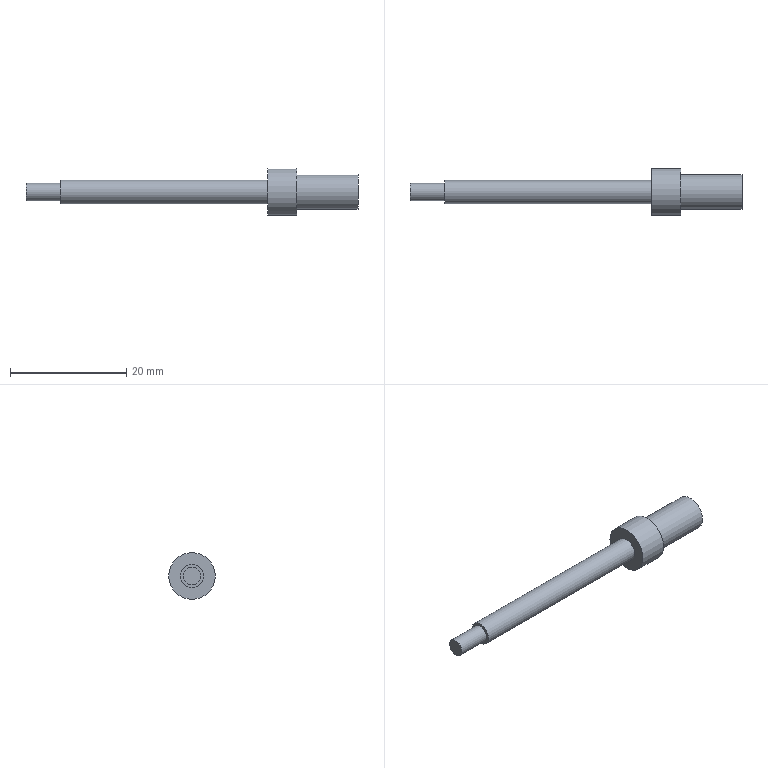Part | STEP file | 1-75.6 | 1 solid | 9 faces | box 57 x 8 x 8 mm | volume 1037 mm3 | plane 5 | cylinder 4 | commonest cylinder face diameters 3 x1 4 x1 6 x1 8 x1
STEP:
#1=CARTESIAN_POINT('',(0.,0.,0.));
#2=DIRECTION('',(0.,0.,1.));
#3=DIRECTION('',(1.,0.,0.));
#4=AXIS2_PLACEMENT_3D('',#1,#2,#3);
#5=CARTESIAN_POINT('',(0.,4.,0.));
#6=VERTEX_POINT('',#5);
#7=CARTESIAN_POINT('',(0.,0.,0.));
#8=DIRECTION('',(1.,0.,0.));
#9=DIRECTION('',(0.,1.,0.));
#10=AXIS2_PLACEMENT_3D('',#7,#8,#9);
#11=CIRCLE('',#10,4.);
#12=CARTESIAN_POINT('',(0.,0.,0.));
#13=DIRECTION('',(1.,0.,0.));
#14=DIRECTION('',(0.,1.,0.));
#15=AXIS2_PLACEMENT_3D('',#12,#13,#14);
#16=CYLINDRICAL_SURFACE('',#15,4.);
#17=CARTESIAN_POINT('',(0.,0.));
#18=DIRECTION('',(1.,0.));
#19=VECTOR('',#18,1.);
#20=LINE('',#17,#19);
#21=(GEOMETRIC_REPRESENTATION_CONTEXT(2)PARAMETRIC_REPRESENTATION_CONTEXT()REPRESENTATION_CONTEXT('',''));
#22=DEFINITIONAL_REPRESENTATION('',(#20),#21);
#23=PCURVE('',#16,#22);
#24=CARTESIAN_POINT('',(0.,-1.072,0.));
#25=DIRECTION('',(1.,0.,0.));
#26=DIRECTION('',(0.,0.,-1.));
#27=AXIS2_PLACEMENT_3D('',#24,#25,#26);
#28=PLANE('',#27);
#29=CARTESIAN_POINT('',(0.,1.072));
#30=DIRECTION('',(0.,1.));
#31=AXIS2_PLACEMENT_2D('',#29,#30);
#32=CIRCLE('',#31,4.);
#33=(GEOMETRIC_REPRESENTATION_CONTEXT(2)PARAMETRIC_REPRESENTATION_CONTEXT()REPRESENTATION_CONTEXT('',''));
#34=DEFINITIONAL_REPRESENTATION('',(#32),#33);
#35=PCURVE('',#28,#34);
#36=SURFACE_CURVE('',#11,(#23,#35),.PCURVE_S1.);
#37=EDGE_CURVE('',#6,#6,#36,.T.);
#38=ORIENTED_EDGE('',*,*,#37,.T.);
#39=CARTESIAN_POINT('',(5.,4.,0.));
#40=VERTEX_POINT('',#39);
#41=CARTESIAN_POINT('',(0.,4.,0.));
#42=DIRECTION('',(1.,0.,0.));
#43=VECTOR('',#42,1.);
#44=LINE('',#41,#43);
#45=CARTESIAN_POINT('',(6.283,0.));
#46=DIRECTION('',(0.,1.));
#47=VECTOR('',#46,1.);
#48=LINE('',#45,#47);
#49=(GEOMETRIC_REPRESENTATION_CONTEXT(2)PARAMETRIC_REPRESENTATION_CONTEXT()REPRESENTATION_CONTEXT('',''));
#50=DEFINITIONAL_REPRESENTATION('',(#48),#49);
#51=PCURVE('',#16,#50);
#52=CARTESIAN_POINT('',(0.,0.));
#53=DIRECTION('',(0.,1.));
#54=VECTOR('',#53,1.);
#55=LINE('',#52,#54);
#56=(GEOMETRIC_REPRESENTATION_CONTEXT(2)PARAMETRIC_REPRESENTATION_CONTEXT()REPRESENTATION_CONTEXT('',''));
#57=DEFINITIONAL_REPRESENTATION('',(#55),#56);
#58=PCURVE('',#16,#57);
#59=SEAM_CURVE('',#44,(#51,#58),.PCURVE_S1.);
#60=EDGE_CURVE('',#6,#40,#59,.T.);
#61=ORIENTED_EDGE('',*,*,#60,.T.);
#62=CARTESIAN_POINT('',(5.,0.,0.));
#63=DIRECTION('',(1.,0.,0.));
#64=DIRECTION('',(0.,1.,0.));
#65=AXIS2_PLACEMENT_3D('',#62,#63,#64);
#66=CIRCLE('',#65,4.);
#67=CARTESIAN_POINT('',(0.,5.));
#68=DIRECTION('',(1.,0.));
#69=VECTOR('',#68,1.);
#70=LINE('',#67,#69);
#71=(GEOMETRIC_REPRESENTATION_CONTEXT(2)PARAMETRIC_REPRESENTATION_CONTEXT()REPRESENTATION_CONTEXT('',''));
#72=DEFINITIONAL_REPRESENTATION('',(#70),#71);
#73=PCURVE('',#16,#72);
#74=CARTESIAN_POINT('',(5.,-1.072,0.));
#75=DIRECTION('',(1.,0.,0.));
#76=DIRECTION('',(0.,0.,-1.));
#77=AXIS2_PLACEMENT_3D('',#74,#75,#76);
#78=PLANE('',#77);
#79=CARTESIAN_POINT('',(0.,1.072));
#80=DIRECTION('',(0.,1.));
#81=AXIS2_PLACEMENT_2D('',#79,#80);
#82=CIRCLE('',#81,4.);
#83=(GEOMETRIC_REPRESENTATION_CONTEXT(2)PARAMETRIC_REPRESENTATION_CONTEXT()REPRESENTATION_CONTEXT('',''));
#84=DEFINITIONAL_REPRESENTATION('',(#82),#83);
#85=PCURVE('',#78,#84);
#86=SURFACE_CURVE('',#66,(#73,#85),.PCURVE_S1.);
#87=EDGE_CURVE('',#40,#40,#86,.T.);
#88=ORIENTED_EDGE('',*,*,#87,.F.);
#89=ORIENTED_EDGE('',*,*,#60,.F.);
#90=EDGE_LOOP('',(#38,#61,#88,#89));
#91=FACE_BOUND('',#90,.T.);
#92=ADVANCED_FACE('',(#91),#16,.T.);
#93=ORIENTED_EDGE('',*,*,#87,.T.);
#94=EDGE_LOOP('',(#93));
#95=FACE_BOUND('',#94,.T.);
#96=CARTESIAN_POINT('',(5.,3.,0.));
#97=VERTEX_POINT('',#96);
#98=CARTESIAN_POINT('',(5.,0.,0.));
#99=DIRECTION('',(1.,0.,0.));
#100=DIRECTION('',(0.,1.,0.));
#101=AXIS2_PLACEMENT_3D('',#98,#99,#100);
#102=CIRCLE('',#101,3.);
#103=CARTESIAN_POINT('',(0.,1.072));
#104=DIRECTION('',(0.,1.));
#105=AXIS2_PLACEMENT_2D('',#103,#104);
#106=CIRCLE('',#105,3.);
#107=(GEOMETRIC_REPRESENTATION_CONTEXT(2)PARAMETRIC_REPRESENTATION_CONTEXT()REPRESENTATION_CONTEXT('',''));
#108=DEFINITIONAL_REPRESENTATION('',(#106),#107);
#109=PCURVE('',#78,#108);
#110=CARTESIAN_POINT('',(5.,0.,0.));
#111=DIRECTION('',(1.,0.,0.));
#112=DIRECTION('',(0.,1.,0.));
#113=AXIS2_PLACEMENT_3D('',#110,#111,#112);
#114=CYLINDRICAL_SURFACE('',#113,3.);
#115=CARTESIAN_POINT('',(0.,0.));
#116=DIRECTION('',(1.,0.));
#117=VECTOR('',#116,1.);
#118=LINE('',#115,#117);
#119=(GEOMETRIC_REPRESENTATION_CONTEXT(2)PARAMETRIC_REPRESENTATION_CONTEXT()REPRESENTATION_CONTEXT('',''));
#120=DEFINITIONAL_REPRESENTATION('',(#118),#119);
#121=PCURVE('',#114,#120);
#122=SURFACE_CURVE('',#102,(#109,#121),.PCURVE_S1.);
#123=EDGE_CURVE('',#97,#97,#122,.T.);
#124=ORIENTED_EDGE('',*,*,#123,.F.);
#125=EDGE_LOOP('',(#124));
#126=FACE_BOUND('',#125,.T.);
#127=ADVANCED_FACE('',(#95,#126),#78,.T.);
#128=ORIENTED_EDGE('',*,*,#123,.T.);
#129=CARTESIAN_POINT('',(15.5,3.,0.));
#130=VERTEX_POINT('',#129);
#131=CARTESIAN_POINT('',(5.,3.,0.));
#132=DIRECTION('',(1.,0.,0.));
#133=VECTOR('',#132,1.);
#134=LINE('',#131,#133);
#135=CARTESIAN_POINT('',(6.283,0.));
#136=DIRECTION('',(0.,1.));
#137=VECTOR('',#136,1.);
#138=LINE('',#135,#137);
#139=(GEOMETRIC_REPRESENTATION_CONTEXT(2)PARAMETRIC_REPRESENTATION_CONTEXT()REPRESENTATION_CONTEXT('',''));
#140=DEFINITIONAL_REPRESENTATION('',(#138),#139);
#141=PCURVE('',#114,#140);
#142=CARTESIAN_POINT('',(0.,0.));
#143=DIRECTION('',(0.,1.));
#144=VECTOR('',#143,1.);
#145=LINE('',#142,#144);
#146=(GEOMETRIC_REPRESENTATION_CONTEXT(2)PARAMETRIC_REPRESENTATION_CONTEXT()REPRESENTATION_CONTEXT('',''));
#147=DEFINITIONAL_REPRESENTATION('',(#145),#146);
#148=PCURVE('',#114,#147);
#149=SEAM_CURVE('',#134,(#141,#148),.PCURVE_S1.);
#150=EDGE_CURVE('',#97,#130,#149,.T.);
#151=ORIENTED_EDGE('',*,*,#150,.T.);
#152=CARTESIAN_POINT('',(15.5,0.,0.));
#153=DIRECTION('',(1.,0.,0.));
#154=DIRECTION('',(0.,1.,0.));
#155=AXIS2_PLACEMENT_3D('',#152,#153,#154);
#156=CIRCLE('',#155,3.);
#157=CARTESIAN_POINT('',(0.,10.5));
#158=DIRECTION('',(1.,0.));
#159=VECTOR('',#158,1.);
#160=LINE('',#157,#159);
#161=(GEOMETRIC_REPRESENTATION_CONTEXT(2)PARAMETRIC_REPRESENTATION_CONTEXT()REPRESENTATION_CONTEXT('',''));
#162=DEFINITIONAL_REPRESENTATION('',(#160),#161);
#163=PCURVE('',#114,#162);
#164=CARTESIAN_POINT('',(15.5,-0.8038,0.));
#165=DIRECTION('',(1.,0.,0.));
#166=DIRECTION('',(0.,0.,-1.));
#167=AXIS2_PLACEMENT_3D('',#164,#165,#166);
#168=PLANE('',#167);
#169=CARTESIAN_POINT('',(0.,0.8038));
#170=DIRECTION('',(0.,1.));
#171=AXIS2_PLACEMENT_2D('',#169,#170);
#172=CIRCLE('',#171,3.);
#173=(GEOMETRIC_REPRESENTATION_CONTEXT(2)PARAMETRIC_REPRESENTATION_CONTEXT()REPRESENTATION_CONTEXT('',''));
#174=DEFINITIONAL_REPRESENTATION('',(#172),#173);
#175=PCURVE('',#168,#174);
#176=SURFACE_CURVE('',#156,(#163,#175),.PCURVE_S1.);
#177=EDGE_CURVE('',#130,#130,#176,.T.);
#178=ORIENTED_EDGE('',*,*,#177,.F.);
#179=ORIENTED_EDGE('',*,*,#150,.F.);
#180=EDGE_LOOP('',(#128,#151,#178,#179));
#181=FACE_BOUND('',#180,.T.);
#182=ADVANCED_FACE('',(#181),#114,.T.);
#183=ORIENTED_EDGE('',*,*,#177,.T.);
#184=EDGE_LOOP('',(#183));
#185=FACE_BOUND('',#184,.T.);
#186=ADVANCED_FACE('',(#185),#168,.T.);
#187=ORIENTED_EDGE('',*,*,#37,.T.);
#188=EDGE_LOOP('',(#187));
#189=FACE_BOUND('',#188,.F.);
#190=CARTESIAN_POINT('',(0.,2.,0.));
#191=VERTEX_POINT('',#190);
#192=CARTESIAN_POINT('',(0.,0.,0.));
#193=DIRECTION('',(1.,0.,0.));
#194=DIRECTION('',(0.,1.,0.));
#195=AXIS2_PLACEMENT_3D('',#192,#193,#194);
#196=CIRCLE('',#195,2.);
#197=CARTESIAN_POINT('',(0.,1.072));
#198=DIRECTION('',(0.,1.));
#199=AXIS2_PLACEMENT_2D('',#197,#198);
#200=CIRCLE('',#199,2.);
#201=(GEOMETRIC_REPRESENTATION_CONTEXT(2)PARAMETRIC_REPRESENTATION_CONTEXT()REPRESENTATION_CONTEXT('',''));
#202=DEFINITIONAL_REPRESENTATION('',(#200),#201);
#203=PCURVE('',#28,#202);
#204=CARTESIAN_POINT('',(0.,0.,0.));
#205=DIRECTION('',(-1.,0.,0.));
#206=DIRECTION('',(0.,1.,0.));
#207=AXIS2_PLACEMENT_3D('',#204,#205,#206);
#208=CYLINDRICAL_SURFACE('',#207,2.);
#209=CARTESIAN_POINT('',(6.283,0.));
#210=DIRECTION('',(-1.,0.));
#211=VECTOR('',#210,1.);
#212=LINE('',#209,#211);
#213=(GEOMETRIC_REPRESENTATION_CONTEXT(2)PARAMETRIC_REPRESENTATION_CONTEXT()REPRESENTATION_CONTEXT('',''));
#214=DEFINITIONAL_REPRESENTATION('',(#212),#213);
#215=PCURVE('',#208,#214);
#216=SURFACE_CURVE('',#196,(#203,#215),.PCURVE_S1.);
#217=EDGE_CURVE('',#191,#191,#216,.T.);
#218=ORIENTED_EDGE('',*,*,#217,.F.);
#219=EDGE_LOOP('',(#218));
#220=FACE_BOUND('',#219,.F.);
#221=ADVANCED_FACE('',(#189,#220),#28,.F.);
#222=CARTESIAN_POINT('',(-35.5,2.,0.));
#223=VERTEX_POINT('',#222);
#224=CARTESIAN_POINT('',(0.,2.,0.));
#225=DIRECTION('',(-1.,0.,0.));
#226=VECTOR('',#225,1.);
#227=LINE('',#224,#226);
#228=CARTESIAN_POINT('',(6.283,0.));
#229=DIRECTION('',(0.,1.));
#230=VECTOR('',#229,1.);
#231=LINE('',#228,#230);
#232=(GEOMETRIC_REPRESENTATION_CONTEXT(2)PARAMETRIC_REPRESENTATION_CONTEXT()REPRESENTATION_CONTEXT('',''));
#233=DEFINITIONAL_REPRESENTATION('',(#231),#232);
#234=PCURVE('',#208,#233);
#235=CARTESIAN_POINT('',(0.,0.));
#236=DIRECTION('',(0.,1.));
#237=VECTOR('',#236,1.);
#238=LINE('',#235,#237);
#239=(GEOMETRIC_REPRESENTATION_CONTEXT(2)PARAMETRIC_REPRESENTATION_CONTEXT()REPRESENTATION_CONTEXT('',''));
#240=DEFINITIONAL_REPRESENTATION('',(#238),#239);
#241=PCURVE('',#208,#240);
#242=SEAM_CURVE('',#227,(#234,#241),.PCURVE_S1.);
#243=EDGE_CURVE('',#191,#223,#242,.T.);
#244=ORIENTED_EDGE('',*,*,#243,.T.);
#245=CARTESIAN_POINT('',(-35.5,0.,0.));
#246=DIRECTION('',(1.,0.,0.));
#247=DIRECTION('',(0.,1.,0.));
#248=AXIS2_PLACEMENT_3D('',#245,#246,#247);
#249=CIRCLE('',#248,2.);
#250=CARTESIAN_POINT('',(6.283,35.5));
#251=DIRECTION('',(-1.,0.));
#252=VECTOR('',#251,1.);
#253=LINE('',#250,#252);
#254=(GEOMETRIC_REPRESENTATION_CONTEXT(2)PARAMETRIC_REPRESENTATION_CONTEXT()REPRESENTATION_CONTEXT('',''));
#255=DEFINITIONAL_REPRESENTATION('',(#253),#254);
#256=PCURVE('',#208,#255);
#257=CARTESIAN_POINT('',(-35.5,-0.5359,0.));
#258=DIRECTION('',(1.,0.,0.));
#259=DIRECTION('',(0.,0.,-1.));
#260=AXIS2_PLACEMENT_3D('',#257,#258,#259);
#261=PLANE('',#260);
#262=CARTESIAN_POINT('',(0.,0.5359));
#263=DIRECTION('',(0.,1.));
#264=AXIS2_PLACEMENT_2D('',#262,#263);
#265=CIRCLE('',#264,2.);
#266=(GEOMETRIC_REPRESENTATION_CONTEXT(2)PARAMETRIC_REPRESENTATION_CONTEXT()REPRESENTATION_CONTEXT('',''));
#267=DEFINITIONAL_REPRESENTATION('',(#265),#266);
#268=PCURVE('',#261,#267);
#269=SURFACE_CURVE('',#249,(#256,#268),.PCURVE_S1.);
#270=EDGE_CURVE('',#223,#223,#269,.T.);
#271=ORIENTED_EDGE('',*,*,#270,.T.);
#272=ORIENTED_EDGE('',*,*,#243,.F.);
#273=ORIENTED_EDGE('',*,*,#217,.F.);
#274=EDGE_LOOP('',(#244,#271,#272,#273));
#275=FACE_BOUND('',#274,.T.);
#276=ADVANCED_FACE('',(#275),#208,.T.);
#277=ORIENTED_EDGE('',*,*,#270,.T.);
#278=EDGE_LOOP('',(#277));
#279=FACE_BOUND('',#278,.F.);
#280=CARTESIAN_POINT('',(-35.5,1.5,0.));
#281=VERTEX_POINT('',#280);
#282=CARTESIAN_POINT('',(-35.5,0.,0.));
#283=DIRECTION('',(1.,0.,0.));
#284=DIRECTION('',(0.,1.,0.));
#285=AXIS2_PLACEMENT_3D('',#282,#283,#284);
#286=CIRCLE('',#285,1.5);
#287=CARTESIAN_POINT('',(0.,0.5359));
#288=DIRECTION('',(0.,1.));
#289=AXIS2_PLACEMENT_2D('',#287,#288);
#290=CIRCLE('',#289,1.5);
#291=(GEOMETRIC_REPRESENTATION_CONTEXT(2)PARAMETRIC_REPRESENTATION_CONTEXT()REPRESENTATION_CONTEXT('',''));
#292=DEFINITIONAL_REPRESENTATION('',(#290),#291);
#293=PCURVE('',#261,#292);
#294=CARTESIAN_POINT('',(-35.5,0.,0.));
#295=DIRECTION('',(-1.,0.,0.));
#296=DIRECTION('',(0.,1.,0.));
#297=AXIS2_PLACEMENT_3D('',#294,#295,#296);
#298=CYLINDRICAL_SURFACE('',#297,1.5);
#299=CARTESIAN_POINT('',(6.283,0.));
#300=DIRECTION('',(-1.,0.));
#301=VECTOR('',#300,1.);
#302=LINE('',#299,#301);
#303=(GEOMETRIC_REPRESENTATION_CONTEXT(2)PARAMETRIC_REPRESENTATION_CONTEXT()REPRESENTATION_CONTEXT('',''));
#304=DEFINITIONAL_REPRESENTATION('',(#302),#303);
#305=PCURVE('',#298,#304);
#306=SURFACE_CURVE('',#286,(#293,#305),.PCURVE_S1.);
#307=EDGE_CURVE('',#281,#281,#306,.T.);
#308=ORIENTED_EDGE('',*,*,#307,.F.);
#309=EDGE_LOOP('',(#308));
#310=FACE_BOUND('',#309,.F.);
#311=ADVANCED_FACE('',(#279,#310),#261,.F.);
#312=CARTESIAN_POINT('',(-41.5,1.5,0.));
#313=VERTEX_POINT('',#312);
#314=CARTESIAN_POINT('',(-35.5,1.5,0.));
#315=DIRECTION('',(-1.,0.,0.));
#316=VECTOR('',#315,1.);
#317=LINE('',#314,#316);
#318=CARTESIAN_POINT('',(6.283,0.));
#319=DIRECTION('',(0.,1.));
#320=VECTOR('',#319,1.);
#321=LINE('',#318,#320);
#322=(GEOMETRIC_REPRESENTATION_CONTEXT(2)PARAMETRIC_REPRESENTATION_CONTEXT()REPRESENTATION_CONTEXT('',''));
#323=DEFINITIONAL_REPRESENTATION('',(#321),#322);
#324=PCURVE('',#298,#323);
#325=CARTESIAN_POINT('',(0.,0.));
#326=DIRECTION('',(0.,1.));
#327=VECTOR('',#326,1.);
#328=LINE('',#325,#327);
#329=(GEOMETRIC_REPRESENTATION_CONTEXT(2)PARAMETRIC_REPRESENTATION_CONTEXT()REPRESENTATION_CONTEXT('',''));
#330=DEFINITIONAL_REPRESENTATION('',(#328),#329);
#331=PCURVE('',#298,#330);
#332=SEAM_CURVE('',#317,(#324,#331),.PCURVE_S1.);
#333=EDGE_CURVE('',#281,#313,#332,.T.);
#334=ORIENTED_EDGE('',*,*,#333,.T.);
#335=CARTESIAN_POINT('',(-41.5,0.,0.));
#336=DIRECTION('',(1.,0.,0.));
#337=DIRECTION('',(0.,1.,0.));
#338=AXIS2_PLACEMENT_3D('',#335,#336,#337);
#339=CIRCLE('',#338,1.5);
#340=CARTESIAN_POINT('',(6.283,6.));
#341=DIRECTION('',(-1.,0.));
#342=VECTOR('',#341,1.);
#343=LINE('',#340,#342);
#344=(GEOMETRIC_REPRESENTATION_CONTEXT(2)PARAMETRIC_REPRESENTATION_CONTEXT()REPRESENTATION_CONTEXT('',''));
#345=DEFINITIONAL_REPRESENTATION('',(#343),#344);
#346=PCURVE('',#298,#345);
#347=CARTESIAN_POINT('',(-41.5,-0.4019,0.));
#348=DIRECTION('',(1.,0.,0.));
#349=DIRECTION('',(0.,0.,-1.));
#350=AXIS2_PLACEMENT_3D('',#347,#348,#349);
#351=PLANE('',#350);
#352=CARTESIAN_POINT('',(0.,0.4019));
#353=DIRECTION('',(0.,1.));
#354=AXIS2_PLACEMENT_2D('',#352,#353);
#355=CIRCLE('',#354,1.5);
#356=(GEOMETRIC_REPRESENTATION_CONTEXT(2)PARAMETRIC_REPRESENTATION_CONTEXT()REPRESENTATION_CONTEXT('',''));
#357=DEFINITIONAL_REPRESENTATION('',(#355),#356);
#358=PCURVE('',#351,#357);
#359=SURFACE_CURVE('',#339,(#346,#358),.PCURVE_S1.);
#360=EDGE_CURVE('',#313,#313,#359,.T.);
#361=ORIENTED_EDGE('',*,*,#360,.T.);
#362=ORIENTED_EDGE('',*,*,#333,.F.);
#363=ORIENTED_EDGE('',*,*,#307,.F.);
#364=EDGE_LOOP('',(#334,#361,#362,#363));
#365=FACE_BOUND('',#364,.T.);
#366=ADVANCED_FACE('',(#365),#298,.T.);
#367=ORIENTED_EDGE('',*,*,#360,.T.);
#368=EDGE_LOOP('',(#367));
#369=FACE_BOUND('',#368,.F.);
#370=ADVANCED_FACE('',(#369),#351,.F.);
#371=CLOSED_SHELL('',(#92,#127,#182,#186,#221,#276,#311,#366,#370));
#372=MANIFOLD_SOLID_BREP('',#371);
#373=(LENGTH_UNIT()NAMED_UNIT(*)SI_UNIT(.MILLI.,.METRE.));
#374=UNCERTAINTY_MEASURE_WITH_UNIT(LENGTH_MEASURE(0.0000001),#373,'','');
#375=(NAMED_UNIT(*)PLANE_ANGLE_UNIT()SI_UNIT($,.RADIAN.));
#376=(NAMED_UNIT(*)SI_UNIT($,.STERADIAN.)SOLID_ANGLE_UNIT());
#377=(GEOMETRIC_REPRESENTATION_CONTEXT(3)GLOBAL_UNCERTAINTY_ASSIGNED_CONTEXT((#374))GLOBAL_UNIT_ASSIGNED_CONTEXT((#373,#375,#376))REPRESENTATION_CONTEXT('',''));
#378=ADVANCED_BREP_SHAPE_REPRESENTATION('',(#4,#372),#377);